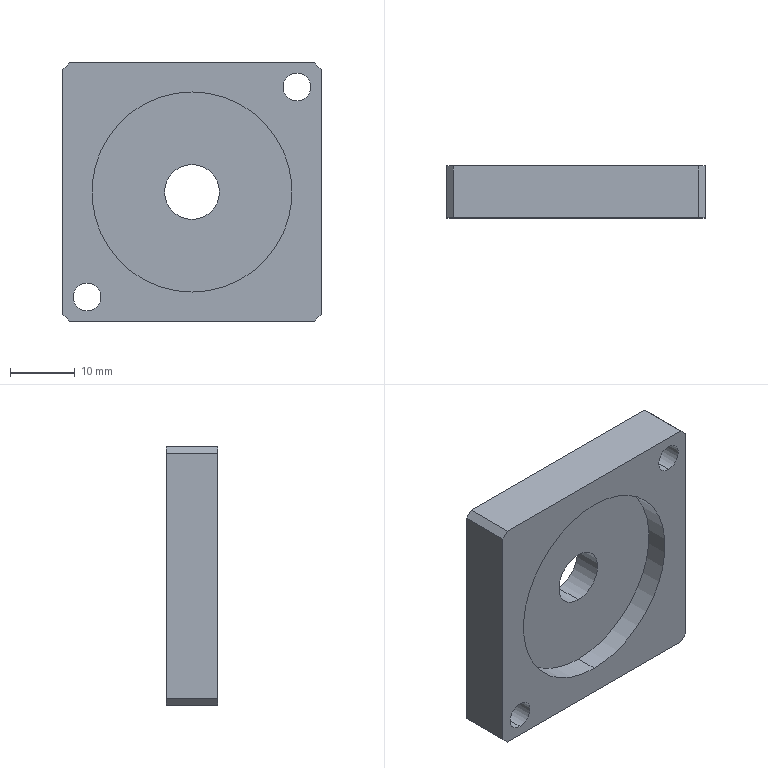Part | SolidWorks | features ICE 2, Chamfer 1, Cut 1, Extrusion 1 | 1 solid | 19 faces | box 40 x 8 x 40 mm | volume 9655 mm3 | plane 11 | cylinder 8 | commonest cylinder face diameters 4.3 x4 8.5 x2 31 x2
STEP:
#1=CARTESIAN_POINT('',(16.263,8.,14.113));
#2=VERTEX_POINT('',#1);
#3=CARTESIAN_POINT('',(16.263,8.,18.413));
#4=VERTEX_POINT('',#3);
#5=CARTESIAN_POINT('',(16.263,8.,16.263));
#6=DIRECTION('',(0.,1.,0.));
#7=DIRECTION('',(0.,0.,1.));
#8=AXIS2_PLACEMENT_3D('',#5,#6,#7);
#9=CIRCLE('',#8,2.15);
#10=EDGE_CURVE('',#2,#4,#9,.T.);
#11=ORIENTED_EDGE('',*,*,#10,.T.);
#12=CARTESIAN_POINT('',(16.263,0.,18.413));
#13=VERTEX_POINT('',#12);
#14=CARTESIAN_POINT('',(16.263,10.,18.413));
#15=DIRECTION('',(0.,-1.,0.));
#16=VECTOR('',#15,1000.);
#17=LINE('',#14,#16);
#18=EDGE_CURVE('',#4,#13,#17,.T.);
#19=ORIENTED_EDGE('',*,*,#18,.T.);
#20=CARTESIAN_POINT('',(16.263,0.,14.113));
#21=VERTEX_POINT('',#20);
#22=CARTESIAN_POINT('',(16.263,0.,16.263));
#23=DIRECTION('',(0.,-1.,0.));
#24=DIRECTION('',(0.,0.,-1.));
#25=AXIS2_PLACEMENT_3D('',#22,#23,#24);
#26=CIRCLE('',#25,2.15);
#27=EDGE_CURVE('',#13,#21,#26,.T.);
#28=ORIENTED_EDGE('',*,*,#27,.T.);
#29=CARTESIAN_POINT('',(16.263,10.,14.113));
#30=DIRECTION('',(0.,-1.,0.));
#31=VECTOR('',#30,1000.);
#32=LINE('',#29,#31);
#33=EDGE_CURVE('',#2,#21,#32,.T.);
#34=ORIENTED_EDGE('',*,*,#33,.F.);
#35=EDGE_LOOP('',(#11,#19,#28,#34));
#36=FACE_OUTER_BOUND('',#35,.T.);
#37=CARTESIAN_POINT('',(16.263,10.,16.263));
#38=DIRECTION('',(0.,-1.,0.));
#39=DIRECTION('',(0.,0.,-1.));
#40=AXIS2_PLACEMENT_3D('',#37,#38,#39);
#41=CYLINDRICAL_SURFACE('',#40,2.15);
#42=ADVANCED_FACE('',(#36),#41,.F.);
#43=CARTESIAN_POINT('',(-16.263,8.,-18.413));
#44=VERTEX_POINT('',#43);
#45=CARTESIAN_POINT('',(-16.263,8.,-14.113));
#46=VERTEX_POINT('',#45);
#47=CARTESIAN_POINT('',(-16.263,8.,-16.263));
#48=DIRECTION('',(0.,1.,0.));
#49=DIRECTION('',(0.,0.,1.));
#50=AXIS2_PLACEMENT_3D('',#47,#48,#49);
#51=CIRCLE('',#50,2.15);
#52=EDGE_CURVE('',#44,#46,#51,.T.);
#53=ORIENTED_EDGE('',*,*,#52,.T.);
#54=CARTESIAN_POINT('',(-16.263,0.,-14.113));
#55=VERTEX_POINT('',#54);
#56=CARTESIAN_POINT('',(-16.263,10.,-14.113));
#57=DIRECTION('',(0.,-1.,0.));
#58=VECTOR('',#57,1000.);
#59=LINE('',#56,#58);
#60=EDGE_CURVE('',#46,#55,#59,.T.);
#61=ORIENTED_EDGE('',*,*,#60,.T.);
#62=CARTESIAN_POINT('',(-16.263,0.,-18.413));
#63=VERTEX_POINT('',#62);
#64=CARTESIAN_POINT('',(-16.263,0.,-16.263));
#65=DIRECTION('',(0.,-1.,0.));
#66=DIRECTION('',(0.,0.,-1.));
#67=AXIS2_PLACEMENT_3D('',#64,#65,#66);
#68=CIRCLE('',#67,2.15);
#69=EDGE_CURVE('',#55,#63,#68,.T.);
#70=ORIENTED_EDGE('',*,*,#69,.T.);
#71=CARTESIAN_POINT('',(-16.263,10.,-18.413));
#72=DIRECTION('',(0.,-1.,0.));
#73=VECTOR('',#72,1000.);
#74=LINE('',#71,#73);
#75=EDGE_CURVE('',#44,#63,#74,.T.);
#76=ORIENTED_EDGE('',*,*,#75,.F.);
#77=EDGE_LOOP('',(#53,#61,#70,#76));
#78=FACE_OUTER_BOUND('',#77,.T.);
#79=CARTESIAN_POINT('',(-16.263,10.,-16.263));
#80=DIRECTION('',(0.,-1.,0.));
#81=DIRECTION('',(0.,0.,-1.));
#82=AXIS2_PLACEMENT_3D('',#79,#80,#81);
#83=CYLINDRICAL_SURFACE('',#82,2.15);
#84=ADVANCED_FACE('',(#78),#83,.F.);
#85=CARTESIAN_POINT('',(0.,3.5,4.25));
#86=VERTEX_POINT('',#85);
#87=CARTESIAN_POINT('',(0.,3.5,-4.25));
#88=VERTEX_POINT('',#87);
#89=CARTESIAN_POINT('',(0.,3.5,0.));
#90=DIRECTION('',(0.,-1.,0.));
#91=DIRECTION('',(0.,0.,-1.));
#92=AXIS2_PLACEMENT_3D('',#89,#90,#91);
#93=CIRCLE('',#92,4.25);
#94=EDGE_CURVE('',#86,#88,#93,.T.);
#95=ORIENTED_EDGE('',*,*,#94,.T.);
#96=CARTESIAN_POINT('',(0.,8.,-4.25));
#97=VERTEX_POINT('',#96);
#98=CARTESIAN_POINT('',(0.,0.,-4.25));
#99=DIRECTION('',(0.,1.,0.));
#100=VECTOR('',#99,1000.);
#101=LINE('',#98,#100);
#102=EDGE_CURVE('',#88,#97,#101,.T.);
#103=ORIENTED_EDGE('',*,*,#102,.T.);
#104=CARTESIAN_POINT('',(0.,8.,4.25));
#105=VERTEX_POINT('',#104);
#106=CARTESIAN_POINT('',(0.,8.,0.));
#107=DIRECTION('',(0.,1.,0.));
#108=DIRECTION('',(0.,0.,1.));
#109=AXIS2_PLACEMENT_3D('',#106,#107,#108);
#110=CIRCLE('',#109,4.25);
#111=EDGE_CURVE('',#97,#105,#110,.T.);
#112=ORIENTED_EDGE('',*,*,#111,.T.);
#113=CARTESIAN_POINT('',(0.,0.,4.25));
#114=DIRECTION('',(0.,1.,0.));
#115=VECTOR('',#114,1000.);
#116=LINE('',#113,#115);
#117=EDGE_CURVE('',#86,#105,#116,.T.);
#118=ORIENTED_EDGE('',*,*,#117,.F.);
#119=EDGE_LOOP('',(#95,#103,#112,#118));
#120=FACE_OUTER_BOUND('',#119,.T.);
#121=CARTESIAN_POINT('',(0.,0.,0.));
#122=DIRECTION('',(0.,1.,0.));
#123=DIRECTION('',(0.,0.,1.));
#124=AXIS2_PLACEMENT_3D('',#121,#122,#123);
#125=CYLINDRICAL_SURFACE('',#124,4.25);
#126=ADVANCED_FACE('',(#120),#125,.F.);
#127=CARTESIAN_POINT('',(0.,3.5,15.5));
#128=VERTEX_POINT('',#127);
#129=CARTESIAN_POINT('',(0.,3.5,-15.5));
#130=VERTEX_POINT('',#129);
#131=CARTESIAN_POINT('',(0.,3.5,0.));
#132=DIRECTION('',(0.,-1.,0.));
#133=DIRECTION('',(0.,0.,-1.));
#134=AXIS2_PLACEMENT_3D('',#131,#132,#133);
#135=CIRCLE('',#134,15.5);
#136=EDGE_CURVE('',#128,#130,#135,.T.);
#137=ORIENTED_EDGE('',*,*,#136,.F.);
#138=CARTESIAN_POINT('',(0.,0.,15.5));
#139=VERTEX_POINT('',#138);
#140=CARTESIAN_POINT('',(0.,3.5,15.5));
#141=DIRECTION('',(0.,-1.,0.));
#142=VECTOR('',#141,1000.);
#143=LINE('',#140,#142);
#144=EDGE_CURVE('',#128,#139,#143,.T.);
#145=ORIENTED_EDGE('',*,*,#144,.T.);
#146=CARTESIAN_POINT('',(0.,0.,-15.5));
#147=VERTEX_POINT('',#146);
#148=CARTESIAN_POINT('',(0.,0.,0.));
#149=DIRECTION('',(0.,-1.,0.));
#150=DIRECTION('',(0.,0.,-1.));
#151=AXIS2_PLACEMENT_3D('',#148,#149,#150);
#152=CIRCLE('',#151,15.5);
#153=EDGE_CURVE('',#139,#147,#152,.T.);
#154=ORIENTED_EDGE('',*,*,#153,.T.);
#155=CARTESIAN_POINT('',(0.,3.5,-15.5));
#156=DIRECTION('',(0.,-1.,0.));
#157=VECTOR('',#156,1000.);
#158=LINE('',#155,#157);
#159=EDGE_CURVE('',#130,#147,#158,.T.);
#160=ORIENTED_EDGE('',*,*,#159,.F.);
#161=EDGE_LOOP('',(#137,#145,#154,#160));
#162=FACE_OUTER_BOUND('',#161,.T.);
#163=CARTESIAN_POINT('',(0.,3.5,0.));
#164=DIRECTION('',(0.,-1.,0.));
#165=DIRECTION('',(0.,0.,-1.));
#166=AXIS2_PLACEMENT_3D('',#163,#164,#165);
#167=CYLINDRICAL_SURFACE('',#166,15.5);
#168=ADVANCED_FACE('',(#162),#167,.F.);
#169=CARTESIAN_POINT('',(20.,8.,19.));
#170=VERTEX_POINT('',#169);
#171=CARTESIAN_POINT('',(20.,8.,-19.));
#172=VERTEX_POINT('',#171);
#173=CARTESIAN_POINT('',(20.,8.,-20.));
#174=DIRECTION('',(0.,0.,-1.));
#175=VECTOR('',#174,1000.);
#176=LINE('',#173,#175);
#177=EDGE_CURVE('',#170,#172,#176,.T.);
#178=ORIENTED_EDGE('',*,*,#177,.F.);
#179=CARTESIAN_POINT('',(20.,0.,19.));
#180=VERTEX_POINT('',#179);
#181=CARTESIAN_POINT('',(20.,8.,19.));
#182=DIRECTION('',(0.,-1.,0.));
#183=VECTOR('',#182,1000.);
#184=LINE('',#181,#183);
#185=EDGE_CURVE('',#170,#180,#184,.T.);
#186=ORIENTED_EDGE('',*,*,#185,.T.);
#187=CARTESIAN_POINT('',(20.,0.,-19.));
#188=VERTEX_POINT('',#187);
#189=CARTESIAN_POINT('',(20.,0.,-20.));
#190=DIRECTION('',(0.,0.,-1.));
#191=VECTOR('',#190,1000.);
#192=LINE('',#189,#191);
#193=EDGE_CURVE('',#180,#188,#192,.T.);
#194=ORIENTED_EDGE('',*,*,#193,.T.);
#195=CARTESIAN_POINT('',(20.,8.,-19.));
#196=DIRECTION('',(0.,1.,0.));
#197=VECTOR('',#196,1000.);
#198=LINE('',#195,#197);
#199=EDGE_CURVE('',#188,#172,#198,.T.);
#200=ORIENTED_EDGE('',*,*,#199,.T.);
#201=EDGE_LOOP('',(#178,#186,#194,#200));
#202=FACE_OUTER_BOUND('',#201,.T.);
#203=CARTESIAN_POINT('',(20.,8.,-20.));
#204=DIRECTION('',(-1.,0.,0.));
#205=DIRECTION('',(0.,0.,1.));
#206=AXIS2_PLACEMENT_3D('',#203,#204,#205);
#207=PLANE('',#206);
#208=ADVANCED_FACE('',(#202),#207,.F.);
#209=CARTESIAN_POINT('',(19.,0.,-20.));
#210=VERTEX_POINT('',#209);
#211=CARTESIAN_POINT('',(-19.,0.,-20.));
#212=VERTEX_POINT('',#211);
#213=CARTESIAN_POINT('',(-20.,0.,-20.));
#214=DIRECTION('',(-1.,0.,0.));
#215=VECTOR('',#214,1000.);
#216=LINE('',#213,#215);
#217=EDGE_CURVE('',#210,#212,#216,.T.);
#218=ORIENTED_EDGE('',*,*,#217,.T.);
#219=CARTESIAN_POINT('',(-19.,8.,-20.));
#220=VERTEX_POINT('',#219);
#221=CARTESIAN_POINT('',(-19.,8.,-20.));
#222=DIRECTION('',(0.,1.,0.));
#223=VECTOR('',#222,1000.);
#224=LINE('',#221,#223);
#225=EDGE_CURVE('',#212,#220,#224,.T.);
#226=ORIENTED_EDGE('',*,*,#225,.T.);
#227=CARTESIAN_POINT('',(19.,8.,-20.));
#228=VERTEX_POINT('',#227);
#229=CARTESIAN_POINT('',(-20.,8.,-20.));
#230=DIRECTION('',(-1.,0.,0.));
#231=VECTOR('',#230,1000.);
#232=LINE('',#229,#231);
#233=EDGE_CURVE('',#228,#220,#232,.T.);
#234=ORIENTED_EDGE('',*,*,#233,.F.);
#235=CARTESIAN_POINT('',(19.,8.,-20.));
#236=DIRECTION('',(0.,-1.,0.));
#237=VECTOR('',#236,1000.);
#238=LINE('',#235,#237);
#239=EDGE_CURVE('',#228,#210,#238,.T.);
#240=ORIENTED_EDGE('',*,*,#239,.T.);
#241=EDGE_LOOP('',(#218,#226,#234,#240));
#242=FACE_OUTER_BOUND('',#241,.T.);
#243=CARTESIAN_POINT('',(-20.,8.,-20.));
#244=DIRECTION('',(0.,0.,1.));
#245=DIRECTION('',(1.,0.,0.));
#246=AXIS2_PLACEMENT_3D('',#243,#244,#245);
#247=PLANE('',#246);
#248=ADVANCED_FACE('',(#242),#247,.F.);
#249=CARTESIAN_POINT('',(-20.,0.,-19.));
#250=VERTEX_POINT('',#249);
#251=CARTESIAN_POINT('',(-20.,0.,19.));
#252=VERTEX_POINT('',#251);
#253=CARTESIAN_POINT('',(-20.,0.,-20.));
#254=DIRECTION('',(0.,0.,1.));
#255=VECTOR('',#254,1000.);
#256=LINE('',#253,#255);
#257=EDGE_CURVE('',#250,#252,#256,.T.);
#258=ORIENTED_EDGE('',*,*,#257,.T.);
#259=CARTESIAN_POINT('',(-20.,8.,19.));
#260=VERTEX_POINT('',#259);
#261=CARTESIAN_POINT('',(-20.,8.,19.));
#262=DIRECTION('',(0.,1.,0.));
#263=VECTOR('',#262,1000.);
#264=LINE('',#261,#263);
#265=EDGE_CURVE('',#252,#260,#264,.T.);
#266=ORIENTED_EDGE('',*,*,#265,.T.);
#267=CARTESIAN_POINT('',(-20.,8.,-19.));
#268=VERTEX_POINT('',#267);
#269=CARTESIAN_POINT('',(-20.,8.,-20.));
#270=DIRECTION('',(0.,0.,1.));
#271=VECTOR('',#270,1000.);
#272=LINE('',#269,#271);
#273=EDGE_CURVE('',#268,#260,#272,.T.);
#274=ORIENTED_EDGE('',*,*,#273,.F.);
#275=CARTESIAN_POINT('',(-20.,8.,-19.));
#276=DIRECTION('',(0.,-1.,0.));
#277=VECTOR('',#276,1000.);
#278=LINE('',#275,#277);
#279=EDGE_CURVE('',#268,#250,#278,.T.);
#280=ORIENTED_EDGE('',*,*,#279,.T.);
#281=EDGE_LOOP('',(#258,#266,#274,#280));
#282=FACE_OUTER_BOUND('',#281,.T.);
#283=CARTESIAN_POINT('',(-20.,8.,-20.));
#284=DIRECTION('',(1.,0.,0.));
#285=DIRECTION('',(0.,0.,-1.));
#286=AXIS2_PLACEMENT_3D('',#283,#284,#285);
#287=PLANE('',#286);
#288=ADVANCED_FACE('',(#282),#287,.F.);
#289=CARTESIAN_POINT('',(-19.,8.,20.));
#290=VERTEX_POINT('',#289);
#291=CARTESIAN_POINT('',(19.,8.,20.));
#292=VERTEX_POINT('',#291);
#293=CARTESIAN_POINT('',(-20.,8.,20.));
#294=DIRECTION('',(1.,0.,0.));
#295=VECTOR('',#294,1000.);
#296=LINE('',#293,#295);
#297=EDGE_CURVE('',#290,#292,#296,.T.);
#298=ORIENTED_EDGE('',*,*,#297,.F.);
#299=CARTESIAN_POINT('',(-19.,0.,20.));
#300=VERTEX_POINT('',#299);
#301=CARTESIAN_POINT('',(-19.,8.,20.));
#302=DIRECTION('',(0.,-1.,0.));
#303=VECTOR('',#302,1000.);
#304=LINE('',#301,#303);
#305=EDGE_CURVE('',#290,#300,#304,.T.);
#306=ORIENTED_EDGE('',*,*,#305,.T.);
#307=CARTESIAN_POINT('',(19.,0.,20.));
#308=VERTEX_POINT('',#307);
#309=CARTESIAN_POINT('',(-20.,0.,20.));
#310=DIRECTION('',(1.,0.,0.));
#311=VECTOR('',#310,1000.);
#312=LINE('',#309,#311);
#313=EDGE_CURVE('',#300,#308,#312,.T.);
#314=ORIENTED_EDGE('',*,*,#313,.T.);
#315=CARTESIAN_POINT('',(19.,8.,20.));
#316=DIRECTION('',(0.,1.,0.));
#317=VECTOR('',#316,1000.);
#318=LINE('',#315,#317);
#319=EDGE_CURVE('',#308,#292,#318,.T.);
#320=ORIENTED_EDGE('',*,*,#319,.T.);
#321=EDGE_LOOP('',(#298,#306,#314,#320));
#322=FACE_OUTER_BOUND('',#321,.T.);
#323=CARTESIAN_POINT('',(-20.,8.,20.));
#324=DIRECTION('',(0.,0.,-1.));
#325=DIRECTION('',(-1.,0.,0.));
#326=AXIS2_PLACEMENT_3D('',#323,#324,#325);
#327=PLANE('',#326);
#328=ADVANCED_FACE('',(#322),#327,.F.);
#329=ORIENTED_EDGE('',*,*,#10,.F.);
#330=CARTESIAN_POINT('',(16.263,8.,16.263));
#331=DIRECTION('',(0.,1.,0.));
#332=DIRECTION('',(0.,0.,1.));
#333=AXIS2_PLACEMENT_3D('',#330,#331,#332);
#334=CIRCLE('',#333,2.15);
#335=EDGE_CURVE('',#4,#2,#334,.T.);
#336=ORIENTED_EDGE('',*,*,#335,.F.);
#337=EDGE_LOOP('',(#329,#336));
#338=FACE_BOUND('',#337,.T.);
#339=ORIENTED_EDGE('',*,*,#52,.F.);
#340=CARTESIAN_POINT('',(-16.263,8.,-16.263));
#341=DIRECTION('',(0.,1.,0.));
#342=DIRECTION('',(0.,0.,1.));
#343=AXIS2_PLACEMENT_3D('',#340,#341,#342);
#344=CIRCLE('',#343,2.15);
#345=EDGE_CURVE('',#46,#44,#344,.T.);
#346=ORIENTED_EDGE('',*,*,#345,.F.);
#347=EDGE_LOOP('',(#339,#346));
#348=FACE_BOUND('',#347,.T.);
#349=CARTESIAN_POINT('',(0.,8.,0.));
#350=DIRECTION('',(0.,1.,0.));
#351=DIRECTION('',(0.,0.,1.));
#352=AXIS2_PLACEMENT_3D('',#349,#350,#351);
#353=CIRCLE('',#352,4.25);
#354=EDGE_CURVE('',#105,#97,#353,.T.);
#355=ORIENTED_EDGE('',*,*,#354,.F.);
#356=ORIENTED_EDGE('',*,*,#111,.F.);
#357=EDGE_LOOP('',(#355,#356));
#358=FACE_BOUND('',#357,.T.);
#359=ORIENTED_EDGE('',*,*,#273,.T.);
#360=CARTESIAN_POINT('',(-19.5,8.,19.5));
#361=DIRECTION('',(0.7071,0.,0.7071));
#362=VECTOR('',#361,1000.);
#363=LINE('',#360,#362);
#364=EDGE_CURVE('',#260,#290,#363,.T.);
#365=ORIENTED_EDGE('',*,*,#364,.T.);
#366=ORIENTED_EDGE('',*,*,#297,.T.);
#367=CARTESIAN_POINT('',(19.5,8.,19.5));
#368=DIRECTION('',(0.7071,0.,-0.7071));
#369=VECTOR('',#368,1000.);
#370=LINE('',#367,#369);
#371=EDGE_CURVE('',#292,#170,#370,.T.);
#372=ORIENTED_EDGE('',*,*,#371,.T.);
#373=ORIENTED_EDGE('',*,*,#177,.T.);
#374=CARTESIAN_POINT('',(19.5,8.,-19.5));
#375=DIRECTION('',(-0.7071,0.,-0.7071));
#376=VECTOR('',#375,1000.);
#377=LINE('',#374,#376);
#378=EDGE_CURVE('',#172,#228,#377,.T.);
#379=ORIENTED_EDGE('',*,*,#378,.T.);
#380=ORIENTED_EDGE('',*,*,#233,.T.);
#381=CARTESIAN_POINT('',(-19.5,8.,-19.5));
#382=DIRECTION('',(-0.7071,0.,0.7071));
#383=VECTOR('',#382,1000.);
#384=LINE('',#381,#383);
#385=EDGE_CURVE('',#220,#268,#384,.T.);
#386=ORIENTED_EDGE('',*,*,#385,.T.);
#387=EDGE_LOOP('',(#359,#365,#366,#372,#373,#379,#380,#386));
#388=FACE_OUTER_BOUND('',#387,.T.);
#389=CARTESIAN_POINT('',(0.,8.,0.));
#390=DIRECTION('',(0.,1.,0.));
#391=DIRECTION('',(0.,0.,1.));
#392=AXIS2_PLACEMENT_3D('',#389,#390,#391);
#393=PLANE('',#392);
#394=ADVANCED_FACE('',(#338,#348,#358,#388),#393,.T.);
#395=CARTESIAN_POINT('',(16.263,0.,16.263));
#396=DIRECTION('',(0.,-1.,0.));
#397=DIRECTION('',(0.,0.,-1.));
#398=AXIS2_PLACEMENT_3D('',#395,#396,#397);
#399=CIRCLE('',#398,2.15);
#400=EDGE_CURVE('',#21,#13,#399,.T.);
#401=ORIENTED_EDGE('',*,*,#400,.F.);
#402=ORIENTED_EDGE('',*,*,#27,.F.);
#403=EDGE_LOOP('',(#401,#402));
#404=FACE_BOUND('',#403,.T.);
#405=CARTESIAN_POINT('',(-16.263,0.,-16.263));
#406=DIRECTION('',(0.,-1.,0.));
#407=DIRECTION('',(0.,0.,-1.));
#408=AXIS2_PLACEMENT_3D('',#405,#406,#407);
#409=CIRCLE('',#408,2.15);
#410=EDGE_CURVE('',#63,#55,#409,.T.);
#411=ORIENTED_EDGE('',*,*,#410,.F.);
#412=ORIENTED_EDGE('',*,*,#69,.F.);
#413=EDGE_LOOP('',(#411,#412));
#414=FACE_BOUND('',#413,.T.);
#415=CARTESIAN_POINT('',(0.,0.,0.));
#416=DIRECTION('',(0.,-1.,0.));
#417=DIRECTION('',(0.,0.,-1.));
#418=AXIS2_PLACEMENT_3D('',#415,#416,#417);
#419=CIRCLE('',#418,15.5);
#420=EDGE_CURVE('',#147,#139,#419,.T.);
#421=ORIENTED_EDGE('',*,*,#420,.F.);
#422=ORIENTED_EDGE('',*,*,#153,.F.);
#423=EDGE_LOOP('',(#421,#422));
#424=FACE_BOUND('',#423,.T.);
#425=ORIENTED_EDGE('',*,*,#313,.F.);
#426=CARTESIAN_POINT('',(-19.,0.,20.));
#427=DIRECTION('',(-0.7071,0.,-0.7071));
#428=VECTOR('',#427,1000.);
#429=LINE('',#426,#428);
#430=EDGE_CURVE('',#300,#252,#429,.T.);
#431=ORIENTED_EDGE('',*,*,#430,.T.);
#432=ORIENTED_EDGE('',*,*,#257,.F.);
#433=CARTESIAN_POINT('',(-20.,0.,-19.));
#434=DIRECTION('',(0.7071,0.,-0.7071));
#435=VECTOR('',#434,1000.);
#436=LINE('',#433,#435);
#437=EDGE_CURVE('',#250,#212,#436,.T.);
#438=ORIENTED_EDGE('',*,*,#437,.T.);
#439=ORIENTED_EDGE('',*,*,#217,.F.);
#440=CARTESIAN_POINT('',(19.,0.,-20.));
#441=DIRECTION('',(0.7071,0.,0.7071));
#442=VECTOR('',#441,1000.);
#443=LINE('',#440,#442);
#444=EDGE_CURVE('',#210,#188,#443,.T.);
#445=ORIENTED_EDGE('',*,*,#444,.T.);
#446=ORIENTED_EDGE('',*,*,#193,.F.);
#447=CARTESIAN_POINT('',(20.,0.,19.));
#448=DIRECTION('',(-0.7071,0.,0.7071));
#449=VECTOR('',#448,1000.);
#450=LINE('',#447,#449);
#451=EDGE_CURVE('',#180,#308,#450,.T.);
#452=ORIENTED_EDGE('',*,*,#451,.T.);
#453=EDGE_LOOP('',(#425,#431,#432,#438,#439,#445,#446,#452));
#454=FACE_OUTER_BOUND('',#453,.T.);
#455=CARTESIAN_POINT('',(0.,0.,0.));
#456=DIRECTION('',(0.,1.,0.));
#457=DIRECTION('',(0.,0.,1.));
#458=AXIS2_PLACEMENT_3D('',#455,#456,#457);
#459=PLANE('',#458);
#460=ADVANCED_FACE('',(#404,#414,#424,#454),#459,.F.);
#461=ORIENTED_EDGE('',*,*,#364,.F.);
#462=ORIENTED_EDGE('',*,*,#265,.F.);
#463=ORIENTED_EDGE('',*,*,#430,.F.);
#464=ORIENTED_EDGE('',*,*,#305,.F.);
#465=EDGE_LOOP('',(#461,#462,#463,#464));
#466=FACE_OUTER_BOUND('',#465,.T.);
#467=CARTESIAN_POINT('',(-19.,8.,20.));
#468=DIRECTION('',(0.7071,0.,-0.7071));
#469=DIRECTION('',(0.,-1.,0.));
#470=AXIS2_PLACEMENT_3D('',#467,#468,#469);
#471=PLANE('',#470);
#472=ADVANCED_FACE('',(#466),#471,.F.);
#473=ORIENTED_EDGE('',*,*,#371,.F.);
#474=ORIENTED_EDGE('',*,*,#319,.F.);
#475=ORIENTED_EDGE('',*,*,#451,.F.);
#476=ORIENTED_EDGE('',*,*,#185,.F.);
#477=EDGE_LOOP('',(#473,#474,#475,#476));
#478=FACE_OUTER_BOUND('',#477,.T.);
#479=CARTESIAN_POINT('',(20.,8.,19.));
#480=DIRECTION('',(-0.7071,0.,-0.7071));
#481=DIRECTION('',(0.,-1.,0.));
#482=AXIS2_PLACEMENT_3D('',#479,#480,#481);
#483=PLANE('',#482);
#484=ADVANCED_FACE('',(#478),#483,.F.);
#485=ORIENTED_EDGE('',*,*,#385,.F.);
#486=ORIENTED_EDGE('',*,*,#225,.F.);
#487=ORIENTED_EDGE('',*,*,#437,.F.);
#488=ORIENTED_EDGE('',*,*,#279,.F.);
#489=EDGE_LOOP('',(#485,#486,#487,#488));
#490=FACE_OUTER_BOUND('',#489,.T.);
#491=CARTESIAN_POINT('',(-20.,8.,-19.));
#492=DIRECTION('',(0.7071,0.,0.7071));
#493=DIRECTION('',(0.,-1.,0.));
#494=AXIS2_PLACEMENT_3D('',#491,#492,#493);
#495=PLANE('',#494);
#496=ADVANCED_FACE('',(#490),#495,.F.);
#497=ORIENTED_EDGE('',*,*,#378,.F.);
#498=ORIENTED_EDGE('',*,*,#199,.F.);
#499=ORIENTED_EDGE('',*,*,#444,.F.);
#500=ORIENTED_EDGE('',*,*,#239,.F.);
#501=EDGE_LOOP('',(#497,#498,#499,#500));
#502=FACE_OUTER_BOUND('',#501,.T.);
#503=CARTESIAN_POINT('',(19.,8.,-20.));
#504=DIRECTION('',(-0.7071,0.,0.7071));
#505=DIRECTION('',(0.,-1.,0.));
#506=AXIS2_PLACEMENT_3D('',#503,#504,#505);
#507=PLANE('',#506);
#508=ADVANCED_FACE('',(#502),#507,.F.);
#509=ORIENTED_EDGE('',*,*,#144,.F.);
#510=CARTESIAN_POINT('',(0.,3.5,0.));
#511=DIRECTION('',(0.,-1.,0.));
#512=DIRECTION('',(0.,0.,-1.));
#513=AXIS2_PLACEMENT_3D('',#510,#511,#512);
#514=CIRCLE('',#513,15.5);
#515=EDGE_CURVE('',#130,#128,#514,.T.);
#516=ORIENTED_EDGE('',*,*,#515,.F.);
#517=ORIENTED_EDGE('',*,*,#159,.T.);
#518=ORIENTED_EDGE('',*,*,#420,.T.);
#519=EDGE_LOOP('',(#509,#516,#517,#518));
#520=FACE_OUTER_BOUND('',#519,.T.);
#521=CARTESIAN_POINT('',(0.,3.5,0.));
#522=DIRECTION('',(0.,-1.,0.));
#523=DIRECTION('',(0.,0.,-1.));
#524=AXIS2_PLACEMENT_3D('',#521,#522,#523);
#525=CYLINDRICAL_SURFACE('',#524,15.5);
#526=ADVANCED_FACE('',(#520),#525,.F.);
#527=ORIENTED_EDGE('',*,*,#94,.F.);
#528=CARTESIAN_POINT('',(0.,3.5,0.));
#529=DIRECTION('',(0.,-1.,0.));
#530=DIRECTION('',(0.,0.,-1.));
#531=AXIS2_PLACEMENT_3D('',#528,#529,#530);
#532=CIRCLE('',#531,4.25);
#533=EDGE_CURVE('',#88,#86,#532,.T.);
#534=ORIENTED_EDGE('',*,*,#533,.F.);
#535=EDGE_LOOP('',(#527,#534));
#536=FACE_BOUND('',#535,.T.);
#537=ORIENTED_EDGE('',*,*,#515,.T.);
#538=ORIENTED_EDGE('',*,*,#136,.T.);
#539=EDGE_LOOP('',(#537,#538));
#540=FACE_OUTER_BOUND('',#539,.T.);
#541=CARTESIAN_POINT('',(0.,3.5,0.));
#542=DIRECTION('',(0.,-1.,0.));
#543=DIRECTION('',(0.,0.,-1.));
#544=AXIS2_PLACEMENT_3D('',#541,#542,#543);
#545=PLANE('',#544);
#546=ADVANCED_FACE('',(#536,#540),#545,.T.);
#547=ORIENTED_EDGE('',*,*,#102,.F.);
#548=ORIENTED_EDGE('',*,*,#533,.T.);
#549=ORIENTED_EDGE('',*,*,#117,.T.);
#550=ORIENTED_EDGE('',*,*,#354,.T.);
#551=EDGE_LOOP('',(#547,#548,#549,#550));
#552=FACE_OUTER_BOUND('',#551,.T.);
#553=CARTESIAN_POINT('',(0.,0.,0.));
#554=DIRECTION('',(0.,1.,0.));
#555=DIRECTION('',(0.,0.,1.));
#556=AXIS2_PLACEMENT_3D('',#553,#554,#555);
#557=CYLINDRICAL_SURFACE('',#556,4.25);
#558=ADVANCED_FACE('',(#552),#557,.F.);
#559=ORIENTED_EDGE('',*,*,#60,.F.);
#560=ORIENTED_EDGE('',*,*,#345,.T.);
#561=ORIENTED_EDGE('',*,*,#75,.T.);
#562=ORIENTED_EDGE('',*,*,#410,.T.);
#563=EDGE_LOOP('',(#559,#560,#561,#562));
#564=FACE_OUTER_BOUND('',#563,.T.);
#565=CARTESIAN_POINT('',(-16.263,10.,-16.263));
#566=DIRECTION('',(0.,-1.,0.));
#567=DIRECTION('',(0.,0.,-1.));
#568=AXIS2_PLACEMENT_3D('',#565,#566,#567);
#569=CYLINDRICAL_SURFACE('',#568,2.15);
#570=ADVANCED_FACE('',(#564),#569,.F.);
#571=ORIENTED_EDGE('',*,*,#18,.F.);
#572=ORIENTED_EDGE('',*,*,#335,.T.);
#573=ORIENTED_EDGE('',*,*,#33,.T.);
#574=ORIENTED_EDGE('',*,*,#400,.T.);
#575=EDGE_LOOP('',(#571,#572,#573,#574));
#576=FACE_OUTER_BOUND('',#575,.T.);
#577=CARTESIAN_POINT('',(16.263,10.,16.263));
#578=DIRECTION('',(0.,-1.,0.));
#579=DIRECTION('',(0.,0.,-1.));
#580=AXIS2_PLACEMENT_3D('',#577,#578,#579);
#581=CYLINDRICAL_SURFACE('',#580,2.15);
#582=ADVANCED_FACE('',(#576),#581,.F.);
#583=CLOSED_SHELL('',(#42,#84,#126,#168,#208,#248,#288,#328,#394,#460,#472,#484,#496,#508,#526,#546,#558,#570,#582));
#584=MANIFOLD_SOLID_BREP('',#583);
#585=CARTESIAN_POINT('',(0.,0.,0.));
#586=DIRECTION('',(0.,0.,1.));
#587=DIRECTION('',(1.,0.,0.));
#588=AXIS2_PLACEMENT_3D('',#585,#586,#587);
#589=(LENGTH_UNIT()NAMED_UNIT(*)SI_UNIT(.MILLI.,.METRE.));
#590=UNCERTAINTY_MEASURE_WITH_UNIT(LENGTH_MEASURE(0.00001),#589,'','');
#591=(NAMED_UNIT(*)PLANE_ANGLE_UNIT()SI_UNIT($,.RADIAN.));
#592=(NAMED_UNIT(*)SI_UNIT($,.STERADIAN.)SOLID_ANGLE_UNIT());
#593=(GEOMETRIC_REPRESENTATION_CONTEXT(3)GLOBAL_UNCERTAINTY_ASSIGNED_CONTEXT((#590))GLOBAL_UNIT_ASSIGNED_CONTEXT((#589,#591,#592))REPRESENTATION_CONTEXT('',''));
#594=ADVANCED_BREP_SHAPE_REPRESENTATION('',(#584,#588),#593);